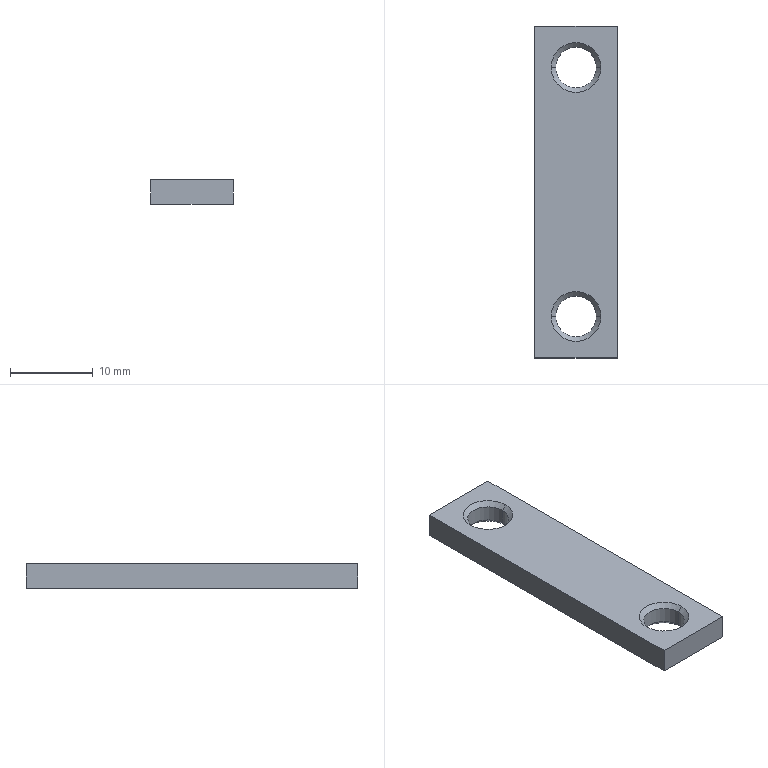Part | STEP file | hhpnt6_2_2_03 | 1 solid | 18 faces | box 10 x 40 x 3 mm | volume 1076 mm3 | cone 8 | plane 6 | cylinder 4 | commonest cylinder face diameters 4.917 x4
STEP:
#1=CARTESIAN_POINT('',(0.,0.,0.));
#2=DIRECTION('',(0.,0.,1.));
#3=DIRECTION('',(1.,0.,0.));
#4=AXIS2_PLACEMENT_3D('',#1,#2,#3);
#5=CARTESIAN_POINT('',(-2.459,-15.,0.5415));
#6=VERTEX_POINT('',#5);
#7=CARTESIAN_POINT('',(-3.,-15.,0.));
#8=VERTEX_POINT('',#7);
#9=CARTESIAN_POINT('',(-3.,-15.,0.));
#10=DIRECTION('',(-0.7071,0.,-0.7071));
#11=VECTOR('',#10,1.);
#12=LINE('',#9,#11);
#13=CARTESIAN_POINT('',(0.,-15.,0.));
#14=DIRECTION('',(0.,0.,-1.));
#15=DIRECTION('',(-1.,0.,0.));
#16=AXIS2_PLACEMENT_3D('',#13,#14,#15);
#17=CONICAL_SURFACE('',#16,3.,0.7854);
#18=CARTESIAN_POINT('',(6.283,0.));
#19=DIRECTION('',(0.,1.));
#20=VECTOR('',#19,1.);
#21=LINE('',#18,#20);
#22=(GEOMETRIC_REPRESENTATION_CONTEXT(2)PARAMETRIC_REPRESENTATION_CONTEXT()REPRESENTATION_CONTEXT('',''));
#23=DEFINITIONAL_REPRESENTATION('',(#21),#22);
#24=PCURVE('',#17,#23);
#25=CARTESIAN_POINT('',(0.,-15.,0.));
#26=DIRECTION('',(0.,0.,-1.));
#27=DIRECTION('',(-1.,0.,0.));
#28=AXIS2_PLACEMENT_3D('',#25,#26,#27);
#29=CONICAL_SURFACE('',#28,3.,0.7854);
#30=CARTESIAN_POINT('',(0.,0.));
#31=DIRECTION('',(0.,1.));
#32=VECTOR('',#31,1.);
#33=LINE('',#30,#32);
#34=(GEOMETRIC_REPRESENTATION_CONTEXT(2)PARAMETRIC_REPRESENTATION_CONTEXT()REPRESENTATION_CONTEXT('',''));
#35=DEFINITIONAL_REPRESENTATION('',(#33),#34);
#36=PCURVE('',#29,#35);
#37=SURFACE_CURVE('',#12,(#24,#36),.PCURVE_S1.);
#38=EDGE_CURVE('',#6,#8,#37,.T.);
#39=ORIENTED_EDGE('',*,*,#38,.T.);
#40=CARTESIAN_POINT('',(3.,-15.,0.));
#41=VERTEX_POINT('',#40);
#42=CARTESIAN_POINT('',(0.,-15.,0.));
#43=DIRECTION('',(0.,0.,-1.));
#44=DIRECTION('',(-1.,0.,0.));
#45=AXIS2_PLACEMENT_3D('',#42,#43,#44);
#46=CIRCLE('',#45,3.);
#47=CARTESIAN_POINT('',(0.,0.));
#48=DIRECTION('',(1.,0.));
#49=VECTOR('',#48,1.);
#50=LINE('',#47,#49);
#51=(GEOMETRIC_REPRESENTATION_CONTEXT(2)PARAMETRIC_REPRESENTATION_CONTEXT()REPRESENTATION_CONTEXT('',''));
#52=DEFINITIONAL_REPRESENTATION('',(#50),#51);
#53=PCURVE('',#17,#52);
#54=CARTESIAN_POINT('',(0.,0.,0.));
#55=DIRECTION('',(0.,0.,1.));
#56=DIRECTION('',(1.,0.,0.));
#57=AXIS2_PLACEMENT_3D('',#54,#55,#56);
#58=PLANE('',#57);
#59=CARTESIAN_POINT('',(-3.,-15.));
#60=CARTESIAN_POINT('',(-3.,-9.804));
#61=CARTESIAN_POINT('',(1.5,-12.402));
#62=CARTESIAN_POINT('',(6.,-15.));
#63=CARTESIAN_POINT('',(1.5,-17.598));
#64=CARTESIAN_POINT('',(-3.,-20.196));
#65=CARTESIAN_POINT('',(-3.,-15.));
#66=(BOUNDED_CURVE()B_SPLINE_CURVE(2,(#59,#60,#61,#62,#63,#64,#65),.UNSPECIFIED.,.T.,.F.)B_SPLINE_CURVE_WITH_KNOTS((1,2,2,2,2,1),(-2.094,0.,2.094,4.189,6.283,8.378),.UNSPECIFIED.)CURVE()GEOMETRIC_REPRESENTATION_ITEM()RATIONAL_B_SPLINE_CURVE((1.,0.5,1.,0.5,1.,0.5,1.))REPRESENTATION_ITEM(''));
#67=(GEOMETRIC_REPRESENTATION_CONTEXT(2)PARAMETRIC_REPRESENTATION_CONTEXT()REPRESENTATION_CONTEXT('',''));
#68=DEFINITIONAL_REPRESENTATION('',(#66),#67);
#69=PCURVE('',#58,#68);
#70=SURFACE_CURVE('',#46,(#53,#69),.PCURVE_S1.);
#71=EDGE_CURVE('',#41,#8,#70,.T.);
#72=ORIENTED_EDGE('',*,*,#71,.F.);
#73=CARTESIAN_POINT('',(2.459,-15.,0.5415));
#74=VERTEX_POINT('',#73);
#75=CARTESIAN_POINT('',(3.,-15.,0.));
#76=DIRECTION('',(0.7071,0.,-0.7071));
#77=VECTOR('',#76,1.);
#78=LINE('',#75,#77);
#79=CARTESIAN_POINT('',(3.142,0.));
#80=DIRECTION('',(0.,1.));
#81=VECTOR('',#80,1.);
#82=LINE('',#79,#81);
#83=(GEOMETRIC_REPRESENTATION_CONTEXT(2)PARAMETRIC_REPRESENTATION_CONTEXT()REPRESENTATION_CONTEXT('',''));
#84=DEFINITIONAL_REPRESENTATION('',(#82),#83);
#85=PCURVE('',#17,#84);
#86=CARTESIAN_POINT('',(3.142,0.));
#87=DIRECTION('',(0.,1.));
#88=VECTOR('',#87,1.);
#89=LINE('',#86,#88);
#90=(GEOMETRIC_REPRESENTATION_CONTEXT(2)PARAMETRIC_REPRESENTATION_CONTEXT()REPRESENTATION_CONTEXT('',''));
#91=DEFINITIONAL_REPRESENTATION('',(#89),#90);
#92=PCURVE('',#29,#91);
#93=SURFACE_CURVE('',#78,(#85,#92),.PCURVE_S1.);
#94=EDGE_CURVE('',#74,#41,#93,.T.);
#95=ORIENTED_EDGE('',*,*,#94,.F.);
#96=CARTESIAN_POINT('',(0.,-15.,0.5415));
#97=DIRECTION('',(0.,0.,-1.));
#98=DIRECTION('',(0.,-1.,0.));
#99=AXIS2_PLACEMENT_3D('',#96,#97,#98);
#100=CIRCLE('',#99,2.459);
#101=CARTESIAN_POINT('',(-1.571,-0.5415));
#102=DIRECTION('',(1.,0.));
#103=VECTOR('',#102,1.);
#104=LINE('',#101,#103);
#105=(GEOMETRIC_REPRESENTATION_CONTEXT(2)PARAMETRIC_REPRESENTATION_CONTEXT()REPRESENTATION_CONTEXT('',''));
#106=DEFINITIONAL_REPRESENTATION('',(#104),#105);
#107=PCURVE('',#17,#106);
#108=CARTESIAN_POINT('',(0.,-15.,1.5));
#109=DIRECTION('',(0.,0.,1.));
#110=DIRECTION('',(1.,0.,0.));
#111=AXIS2_PLACEMENT_3D('',#108,#109,#110);
#112=CYLINDRICAL_SURFACE('',#111,2.458);
#113=CARTESIAN_POINT('',(10.996,-0.9585));
#114=DIRECTION('',(-1.,0.));
#115=VECTOR('',#114,1.);
#116=LINE('',#113,#115);
#117=(GEOMETRIC_REPRESENTATION_CONTEXT(2)PARAMETRIC_REPRESENTATION_CONTEXT()REPRESENTATION_CONTEXT('',''));
#118=DEFINITIONAL_REPRESENTATION('',(#116),#117);
#119=PCURVE('',#112,#118);
#120=SURFACE_CURVE('',#100,(#107,#119),.PCURVE_S1.);
#121=EDGE_CURVE('',#74,#6,#120,.T.);
#122=ORIENTED_EDGE('',*,*,#121,.T.);
#123=EDGE_LOOP('',(#39,#72,#95,#122));
#124=FACE_BOUND('',#123,.F.);
#125=ADVANCED_FACE('',(#124),#17,.F.);
#126=CARTESIAN_POINT('',(-2.459,15.,0.5415));
#127=VERTEX_POINT('',#126);
#128=CARTESIAN_POINT('',(-3.,15.,0.));
#129=VERTEX_POINT('',#128);
#130=CARTESIAN_POINT('',(-3.,15.,0.));
#131=DIRECTION('',(-0.7071,0.,-0.7071));
#132=VECTOR('',#131,1.);
#133=LINE('',#130,#132);
#134=CARTESIAN_POINT('',(0.,15.,0.));
#135=DIRECTION('',(0.,0.,-1.));
#136=DIRECTION('',(-1.,0.,0.));
#137=AXIS2_PLACEMENT_3D('',#134,#135,#136);
#138=CONICAL_SURFACE('',#137,3.,0.7854);
#139=CARTESIAN_POINT('',(6.283,0.));
#140=DIRECTION('',(0.,1.));
#141=VECTOR('',#140,1.);
#142=LINE('',#139,#141);
#143=(GEOMETRIC_REPRESENTATION_CONTEXT(2)PARAMETRIC_REPRESENTATION_CONTEXT()REPRESENTATION_CONTEXT('',''));
#144=DEFINITIONAL_REPRESENTATION('',(#142),#143);
#145=PCURVE('',#138,#144);
#146=CARTESIAN_POINT('',(0.,15.,0.));
#147=DIRECTION('',(0.,0.,-1.));
#148=DIRECTION('',(-1.,0.,0.));
#149=AXIS2_PLACEMENT_3D('',#146,#147,#148);
#150=CONICAL_SURFACE('',#149,3.,0.7854);
#151=CARTESIAN_POINT('',(0.,0.));
#152=DIRECTION('',(0.,1.));
#153=VECTOR('',#152,1.);
#154=LINE('',#151,#153);
#155=(GEOMETRIC_REPRESENTATION_CONTEXT(2)PARAMETRIC_REPRESENTATION_CONTEXT()REPRESENTATION_CONTEXT('',''));
#156=DEFINITIONAL_REPRESENTATION('',(#154),#155);
#157=PCURVE('',#150,#156);
#158=SURFACE_CURVE('',#133,(#145,#157),.PCURVE_S1.);
#159=EDGE_CURVE('',#127,#129,#158,.T.);
#160=ORIENTED_EDGE('',*,*,#159,.T.);
#161=CARTESIAN_POINT('',(3.,15.,0.));
#162=VERTEX_POINT('',#161);
#163=CARTESIAN_POINT('',(0.,15.,0.));
#164=DIRECTION('',(0.,0.,-1.));
#165=DIRECTION('',(-1.,0.,0.));
#166=AXIS2_PLACEMENT_3D('',#163,#164,#165);
#167=CIRCLE('',#166,3.);
#168=CARTESIAN_POINT('',(0.,0.));
#169=DIRECTION('',(1.,0.));
#170=VECTOR('',#169,1.);
#171=LINE('',#168,#170);
#172=(GEOMETRIC_REPRESENTATION_CONTEXT(2)PARAMETRIC_REPRESENTATION_CONTEXT()REPRESENTATION_CONTEXT('',''));
#173=DEFINITIONAL_REPRESENTATION('',(#171),#172);
#174=PCURVE('',#138,#173);
#175=CARTESIAN_POINT('',(-3.,15.));
#176=CARTESIAN_POINT('',(-3.,20.196));
#177=CARTESIAN_POINT('',(1.5,17.598));
#178=CARTESIAN_POINT('',(6.,15.));
#179=CARTESIAN_POINT('',(1.5,12.402));
#180=CARTESIAN_POINT('',(-3.,9.804));
#181=CARTESIAN_POINT('',(-3.,15.));
#182=(BOUNDED_CURVE()B_SPLINE_CURVE(2,(#175,#176,#177,#178,#179,#180,#181),.UNSPECIFIED.,.T.,.F.)B_SPLINE_CURVE_WITH_KNOTS((1,2,2,2,2,1),(-2.094,0.,2.094,4.189,6.283,8.378),.UNSPECIFIED.)CURVE()GEOMETRIC_REPRESENTATION_ITEM()RATIONAL_B_SPLINE_CURVE((1.,0.5,1.,0.5,1.,0.5,1.))REPRESENTATION_ITEM(''));
#183=(GEOMETRIC_REPRESENTATION_CONTEXT(2)PARAMETRIC_REPRESENTATION_CONTEXT()REPRESENTATION_CONTEXT('',''));
#184=DEFINITIONAL_REPRESENTATION('',(#182),#183);
#185=PCURVE('',#58,#184);
#186=SURFACE_CURVE('',#167,(#174,#185),.PCURVE_S1.);
#187=EDGE_CURVE('',#162,#129,#186,.T.);
#188=ORIENTED_EDGE('',*,*,#187,.F.);
#189=CARTESIAN_POINT('',(2.459,15.,0.5415));
#190=VERTEX_POINT('',#189);
#191=CARTESIAN_POINT('',(3.,15.,0.));
#192=DIRECTION('',(0.7071,0.,-0.7071));
#193=VECTOR('',#192,1.);
#194=LINE('',#191,#193);
#195=CARTESIAN_POINT('',(3.142,0.));
#196=DIRECTION('',(0.,1.));
#197=VECTOR('',#196,1.);
#198=LINE('',#195,#197);
#199=(GEOMETRIC_REPRESENTATION_CONTEXT(2)PARAMETRIC_REPRESENTATION_CONTEXT()REPRESENTATION_CONTEXT('',''));
#200=DEFINITIONAL_REPRESENTATION('',(#198),#199);
#201=PCURVE('',#138,#200);
#202=CARTESIAN_POINT('',(3.142,0.));
#203=DIRECTION('',(0.,1.));
#204=VECTOR('',#203,1.);
#205=LINE('',#202,#204);
#206=(GEOMETRIC_REPRESENTATION_CONTEXT(2)PARAMETRIC_REPRESENTATION_CONTEXT()REPRESENTATION_CONTEXT('',''));
#207=DEFINITIONAL_REPRESENTATION('',(#205),#206);
#208=PCURVE('',#150,#207);
#209=SURFACE_CURVE('',#194,(#201,#208),.PCURVE_S1.);
#210=EDGE_CURVE('',#190,#162,#209,.T.);
#211=ORIENTED_EDGE('',*,*,#210,.F.);
#212=CARTESIAN_POINT('',(0.,15.,0.5415));
#213=DIRECTION('',(0.,0.,-1.));
#214=DIRECTION('',(0.,-1.,0.));
#215=AXIS2_PLACEMENT_3D('',#212,#213,#214);
#216=CIRCLE('',#215,2.459);
#217=CARTESIAN_POINT('',(-1.571,-0.5415));
#218=DIRECTION('',(1.,0.));
#219=VECTOR('',#218,1.);
#220=LINE('',#217,#219);
#221=(GEOMETRIC_REPRESENTATION_CONTEXT(2)PARAMETRIC_REPRESENTATION_CONTEXT()REPRESENTATION_CONTEXT('',''));
#222=DEFINITIONAL_REPRESENTATION('',(#220),#221);
#223=PCURVE('',#138,#222);
#224=CARTESIAN_POINT('',(0.,15.,1.5));
#225=DIRECTION('',(0.,0.,1.));
#226=DIRECTION('',(1.,0.,0.));
#227=AXIS2_PLACEMENT_3D('',#224,#225,#226);
#228=CYLINDRICAL_SURFACE('',#227,2.458);
#229=CARTESIAN_POINT('',(10.996,-0.9585));
#230=DIRECTION('',(-1.,0.));
#231=VECTOR('',#230,1.);
#232=LINE('',#229,#231);
#233=(GEOMETRIC_REPRESENTATION_CONTEXT(2)PARAMETRIC_REPRESENTATION_CONTEXT()REPRESENTATION_CONTEXT('',''));
#234=DEFINITIONAL_REPRESENTATION('',(#232),#233);
#235=PCURVE('',#228,#234);
#236=SURFACE_CURVE('',#216,(#223,#235),.PCURVE_S1.);
#237=EDGE_CURVE('',#190,#127,#236,.T.);
#238=ORIENTED_EDGE('',*,*,#237,.T.);
#239=EDGE_LOOP('',(#160,#188,#211,#238));
#240=FACE_BOUND('',#239,.F.);
#241=ADVANCED_FACE('',(#240),#138,.F.);
#242=CARTESIAN_POINT('',(2.458,-15.,2.458));
#243=VERTEX_POINT('',#242);
#244=CARTESIAN_POINT('',(2.458,-15.,1.5));
#245=DIRECTION('',(0.,0.,1.));
#246=VECTOR('',#245,1.);
#247=LINE('',#244,#246);
#248=CARTESIAN_POINT('',(6.283,0.));
#249=DIRECTION('',(0.,1.));
#250=VECTOR('',#249,1.);
#251=LINE('',#248,#250);
#252=(GEOMETRIC_REPRESENTATION_CONTEXT(2)PARAMETRIC_REPRESENTATION_CONTEXT()REPRESENTATION_CONTEXT('',''));
#253=DEFINITIONAL_REPRESENTATION('',(#251),#252);
#254=PCURVE('',#112,#253);
#255=CARTESIAN_POINT('',(0.,-15.,1.5));
#256=DIRECTION('',(0.,0.,1.));
#257=DIRECTION('',(1.,0.,0.));
#258=AXIS2_PLACEMENT_3D('',#255,#256,#257);
#259=CYLINDRICAL_SURFACE('',#258,2.458);
#260=CARTESIAN_POINT('',(0.,0.));
#261=DIRECTION('',(0.,1.));
#262=VECTOR('',#261,1.);
#263=LINE('',#260,#262);
#264=(GEOMETRIC_REPRESENTATION_CONTEXT(2)PARAMETRIC_REPRESENTATION_CONTEXT()REPRESENTATION_CONTEXT('',''));
#265=DEFINITIONAL_REPRESENTATION('',(#263),#264);
#266=PCURVE('',#259,#265);
#267=SURFACE_CURVE('',#247,(#254,#266),.PCURVE_S1.);
#268=EDGE_CURVE('',#74,#243,#267,.T.);
#269=ORIENTED_EDGE('',*,*,#268,.T.);
#270=CARTESIAN_POINT('',(-2.458,-15.,2.458));
#271=VERTEX_POINT('',#270);
#272=CARTESIAN_POINT('',(0.,-15.,2.458));
#273=DIRECTION('',(0.,0.,-1.));
#274=DIRECTION('',(1.,0.,0.));
#275=AXIS2_PLACEMENT_3D('',#272,#273,#274);
#276=CIRCLE('',#275,2.458);
#277=CARTESIAN_POINT('',(6.283,0.9585));
#278=DIRECTION('',(-1.,0.));
#279=VECTOR('',#278,1.);
#280=LINE('',#277,#279);
#281=(GEOMETRIC_REPRESENTATION_CONTEXT(2)PARAMETRIC_REPRESENTATION_CONTEXT()REPRESENTATION_CONTEXT('',''));
#282=DEFINITIONAL_REPRESENTATION('',(#280),#281);
#283=PCURVE('',#112,#282);
#284=CARTESIAN_POINT('',(0.,-15.,3.));
#285=DIRECTION('',(0.,0.,1.));
#286=DIRECTION('',(1.,0.,0.));
#287=AXIS2_PLACEMENT_3D('',#284,#285,#286);
#288=CONICAL_SURFACE('',#287,3.,0.7854);
#289=CARTESIAN_POINT('',(6.283,-0.5415));
#290=DIRECTION('',(-1.,0.));
#291=VECTOR('',#290,1.);
#292=LINE('',#289,#291);
#293=(GEOMETRIC_REPRESENTATION_CONTEXT(2)PARAMETRIC_REPRESENTATION_CONTEXT()REPRESENTATION_CONTEXT('',''));
#294=DEFINITIONAL_REPRESENTATION('',(#292),#293);
#295=PCURVE('',#288,#294);
#296=SURFACE_CURVE('',#276,(#283,#295),.PCURVE_S1.);
#297=EDGE_CURVE('',#243,#271,#296,.T.);
#298=ORIENTED_EDGE('',*,*,#297,.T.);
#299=CARTESIAN_POINT('',(-2.458,-15.,1.5));
#300=DIRECTION('',(0.,0.,1.));
#301=VECTOR('',#300,1.);
#302=LINE('',#299,#301);
#303=CARTESIAN_POINT('',(3.142,0.));
#304=DIRECTION('',(0.,1.));
#305=VECTOR('',#304,1.);
#306=LINE('',#303,#305);
#307=(GEOMETRIC_REPRESENTATION_CONTEXT(2)PARAMETRIC_REPRESENTATION_CONTEXT()REPRESENTATION_CONTEXT('',''));
#308=DEFINITIONAL_REPRESENTATION('',(#306),#307);
#309=PCURVE('',#112,#308);
#310=CARTESIAN_POINT('',(3.142,0.));
#311=DIRECTION('',(0.,1.));
#312=VECTOR('',#311,1.);
#313=LINE('',#310,#312);
#314=(GEOMETRIC_REPRESENTATION_CONTEXT(2)PARAMETRIC_REPRESENTATION_CONTEXT()REPRESENTATION_CONTEXT('',''));
#315=DEFINITIONAL_REPRESENTATION('',(#313),#314);
#316=PCURVE('',#259,#315);
#317=SURFACE_CURVE('',#302,(#309,#316),.PCURVE_S1.);
#318=EDGE_CURVE('',#6,#271,#317,.T.);
#319=ORIENTED_EDGE('',*,*,#318,.F.);
#320=ORIENTED_EDGE('',*,*,#121,.F.);
#321=EDGE_LOOP('',(#269,#298,#319,#320));
#322=FACE_BOUND('',#321,.F.);
#323=ADVANCED_FACE('',(#322),#112,.F.);
#324=CARTESIAN_POINT('',(2.458,15.,2.458));
#325=VERTEX_POINT('',#324);
#326=CARTESIAN_POINT('',(2.458,15.,1.5));
#327=DIRECTION('',(0.,0.,1.));
#328=VECTOR('',#327,1.);
#329=LINE('',#326,#328);
#330=CARTESIAN_POINT('',(6.283,0.));
#331=DIRECTION('',(0.,1.));
#332=VECTOR('',#331,1.);
#333=LINE('',#330,#332);
#334=(GEOMETRIC_REPRESENTATION_CONTEXT(2)PARAMETRIC_REPRESENTATION_CONTEXT()REPRESENTATION_CONTEXT('',''));
#335=DEFINITIONAL_REPRESENTATION('',(#333),#334);
#336=PCURVE('',#228,#335);
#337=CARTESIAN_POINT('',(0.,15.,1.5));
#338=DIRECTION('',(0.,0.,1.));
#339=DIRECTION('',(1.,0.,0.));
#340=AXIS2_PLACEMENT_3D('',#337,#338,#339);
#341=CYLINDRICAL_SURFACE('',#340,2.458);
#342=CARTESIAN_POINT('',(0.,0.));
#343=DIRECTION('',(0.,1.));
#344=VECTOR('',#343,1.);
#345=LINE('',#342,#344);
#346=(GEOMETRIC_REPRESENTATION_CONTEXT(2)PARAMETRIC_REPRESENTATION_CONTEXT()REPRESENTATION_CONTEXT('',''));
#347=DEFINITIONAL_REPRESENTATION('',(#345),#346);
#348=PCURVE('',#341,#347);
#349=SURFACE_CURVE('',#329,(#336,#348),.PCURVE_S1.);
#350=EDGE_CURVE('',#190,#325,#349,.T.);
#351=ORIENTED_EDGE('',*,*,#350,.T.);
#352=CARTESIAN_POINT('',(-2.458,15.,2.458));
#353=VERTEX_POINT('',#352);
#354=CARTESIAN_POINT('',(0.,15.,2.458));
#355=DIRECTION('',(0.,0.,-1.));
#356=DIRECTION('',(1.,0.,0.));
#357=AXIS2_PLACEMENT_3D('',#354,#355,#356);
#358=CIRCLE('',#357,2.458);
#359=CARTESIAN_POINT('',(6.283,0.9585));
#360=DIRECTION('',(-1.,0.));
#361=VECTOR('',#360,1.);
#362=LINE('',#359,#361);
#363=(GEOMETRIC_REPRESENTATION_CONTEXT(2)PARAMETRIC_REPRESENTATION_CONTEXT()REPRESENTATION_CONTEXT('',''));
#364=DEFINITIONAL_REPRESENTATION('',(#362),#363);
#365=PCURVE('',#228,#364);
#366=CARTESIAN_POINT('',(0.,15.,3.));
#367=DIRECTION('',(0.,0.,1.));
#368=DIRECTION('',(1.,0.,0.));
#369=AXIS2_PLACEMENT_3D('',#366,#367,#368);
#370=CONICAL_SURFACE('',#369,3.,0.7854);
#371=CARTESIAN_POINT('',(6.283,-0.5415));
#372=DIRECTION('',(-1.,0.));
#373=VECTOR('',#372,1.);
#374=LINE('',#371,#373);
#375=(GEOMETRIC_REPRESENTATION_CONTEXT(2)PARAMETRIC_REPRESENTATION_CONTEXT()REPRESENTATION_CONTEXT('',''));
#376=DEFINITIONAL_REPRESENTATION('',(#374),#375);
#377=PCURVE('',#370,#376);
#378=SURFACE_CURVE('',#358,(#365,#377),.PCURVE_S1.);
#379=EDGE_CURVE('',#325,#353,#378,.T.);
#380=ORIENTED_EDGE('',*,*,#379,.T.);
#381=CARTESIAN_POINT('',(-2.458,15.,1.5));
#382=DIRECTION('',(0.,0.,1.));
#383=VECTOR('',#382,1.);
#384=LINE('',#381,#383);
#385=CARTESIAN_POINT('',(3.142,0.));
#386=DIRECTION('',(0.,1.));
#387=VECTOR('',#386,1.);
#388=LINE('',#385,#387);
#389=(GEOMETRIC_REPRESENTATION_CONTEXT(2)PARAMETRIC_REPRESENTATION_CONTEXT()REPRESENTATION_CONTEXT('',''));
#390=DEFINITIONAL_REPRESENTATION('',(#388),#389);
#391=PCURVE('',#228,#390);
#392=CARTESIAN_POINT('',(3.142,0.));
#393=DIRECTION('',(0.,1.));
#394=VECTOR('',#393,1.);
#395=LINE('',#392,#394);
#396=(GEOMETRIC_REPRESENTATION_CONTEXT(2)PARAMETRIC_REPRESENTATION_CONTEXT()REPRESENTATION_CONTEXT('',''));
#397=DEFINITIONAL_REPRESENTATION('',(#395),#396);
#398=PCURVE('',#341,#397);
#399=SURFACE_CURVE('',#384,(#391,#398),.PCURVE_S1.);
#400=EDGE_CURVE('',#127,#353,#399,.T.);
#401=ORIENTED_EDGE('',*,*,#400,.F.);
#402=ORIENTED_EDGE('',*,*,#237,.F.);
#403=EDGE_LOOP('',(#351,#380,#401,#402));
#404=FACE_BOUND('',#403,.F.);
#405=ADVANCED_FACE('',(#404),#228,.F.);
#406=CARTESIAN_POINT('',(3.,-15.,3.));
#407=VERTEX_POINT('',#406);
#408=CARTESIAN_POINT('',(3.,-15.,3.));
#409=DIRECTION('',(0.7071,0.,0.7071));
#410=VECTOR('',#409,1.);
#411=LINE('',#408,#410);
#412=CARTESIAN_POINT('',(6.283,0.));
#413=DIRECTION('',(0.,1.));
#414=VECTOR('',#413,1.);
#415=LINE('',#412,#414);
#416=(GEOMETRIC_REPRESENTATION_CONTEXT(2)PARAMETRIC_REPRESENTATION_CONTEXT()REPRESENTATION_CONTEXT('',''));
#417=DEFINITIONAL_REPRESENTATION('',(#415),#416);
#418=PCURVE('',#288,#417);
#419=CARTESIAN_POINT('',(0.,-15.,3.));
#420=DIRECTION('',(0.,0.,1.));
#421=DIRECTION('',(1.,0.,0.));
#422=AXIS2_PLACEMENT_3D('',#419,#420,#421);
#423=CONICAL_SURFACE('',#422,3.,0.7854);
#424=CARTESIAN_POINT('',(0.,0.));
#425=DIRECTION('',(0.,1.));
#426=VECTOR('',#425,1.);
#427=LINE('',#424,#426);
#428=(GEOMETRIC_REPRESENTATION_CONTEXT(2)PARAMETRIC_REPRESENTATION_CONTEXT()REPRESENTATION_CONTEXT('',''));
#429=DEFINITIONAL_REPRESENTATION('',(#427),#428);
#430=PCURVE('',#423,#429);
#431=SURFACE_CURVE('',#411,(#418,#430),.PCURVE_S1.);
#432=EDGE_CURVE('',#243,#407,#431,.T.);
#433=ORIENTED_EDGE('',*,*,#432,.T.);
#434=CARTESIAN_POINT('',(-3.,-15.,3.));
#435=VERTEX_POINT('',#434);
#436=CARTESIAN_POINT('',(0.,-15.,3.));
#437=DIRECTION('',(0.,0.,-1.));
#438=DIRECTION('',(1.,0.,0.));
#439=AXIS2_PLACEMENT_3D('',#436,#437,#438);
#440=CIRCLE('',#439,3.);
#441=CARTESIAN_POINT('',(6.283,0.));
#442=DIRECTION('',(-1.,0.));
#443=VECTOR('',#442,1.);
#444=LINE('',#441,#443);
#445=(GEOMETRIC_REPRESENTATION_CONTEXT(2)PARAMETRIC_REPRESENTATION_CONTEXT()REPRESENTATION_CONTEXT('',''));
#446=DEFINITIONAL_REPRESENTATION('',(#444),#445);
#447=PCURVE('',#288,#446);
#448=CARTESIAN_POINT('',(0.,0.,3.));
#449=DIRECTION('',(0.,0.,1.));
#450=DIRECTION('',(1.,0.,0.));
#451=AXIS2_PLACEMENT_3D('',#448,#449,#450);
#452=PLANE('',#451);
#453=CARTESIAN_POINT('',(3.,-15.));
#454=CARTESIAN_POINT('',(3.,-20.196));
#455=CARTESIAN_POINT('',(-1.5,-17.598));
#456=CARTESIAN_POINT('',(-6.,-15.));
#457=CARTESIAN_POINT('',(-1.5,-12.402));
#458=CARTESIAN_POINT('',(3.,-9.804));
#459=CARTESIAN_POINT('',(3.,-15.));
#460=(BOUNDED_CURVE()B_SPLINE_CURVE(2,(#453,#454,#455,#456,#457,#458,#459),.UNSPECIFIED.,.T.,.F.)B_SPLINE_CURVE_WITH_KNOTS((1,2,2,2,2,1),(-2.094,0.,2.094,4.189,6.283,8.378),.UNSPECIFIED.)CURVE()GEOMETRIC_REPRESENTATION_ITEM()RATIONAL_B_SPLINE_CURVE((1.,0.5,1.,0.5,1.,0.5,1.))REPRESENTATION_ITEM(''));
#461=(GEOMETRIC_REPRESENTATION_CONTEXT(2)PARAMETRIC_REPRESENTATION_CONTEXT()REPRESENTATION_CONTEXT('',''));
#462=DEFINITIONAL_REPRESENTATION('',(#460),#461);
#463=PCURVE('',#452,#462);
#464=SURFACE_CURVE('',#440,(#447,#463),.PCURVE_S1.);
#465=EDGE_CURVE('',#407,#435,#464,.T.);
#466=ORIENTED_EDGE('',*,*,#465,.T.);
#467=CARTESIAN_POINT('',(-3.,-15.,3.));
#468=DIRECTION('',(-0.7071,0.,0.7071));
#469=VECTOR('',#468,1.);
#470=LINE('',#467,#469);
#471=CARTESIAN_POINT('',(3.142,0.));
#472=DIRECTION('',(0.,1.));
#473=VECTOR('',#472,1.);
#474=LINE('',#471,#473);
#475=(GEOMETRIC_REPRESENTATION_CONTEXT(2)PARAMETRIC_REPRESENTATION_CONTEXT()REPRESENTATION_CONTEXT('',''));
#476=DEFINITIONAL_REPRESENTATION('',(#474),#475);
#477=PCURVE('',#288,#476);
#478=CARTESIAN_POINT('',(3.142,0.));
#479=DIRECTION('',(0.,1.));
#480=VECTOR('',#479,1.);
#481=LINE('',#478,#480);
#482=(GEOMETRIC_REPRESENTATION_CONTEXT(2)PARAMETRIC_REPRESENTATION_CONTEXT()REPRESENTATION_CONTEXT('',''));
#483=DEFINITIONAL_REPRESENTATION('',(#481),#482);
#484=PCURVE('',#423,#483);
#485=SURFACE_CURVE('',#470,(#477,#484),.PCURVE_S1.);
#486=EDGE_CURVE('',#271,#435,#485,.T.);
#487=ORIENTED_EDGE('',*,*,#486,.F.);
#488=ORIENTED_EDGE('',*,*,#297,.F.);
#489=EDGE_LOOP('',(#433,#466,#487,#488));
#490=FACE_BOUND('',#489,.F.);
#491=ADVANCED_FACE('',(#490),#288,.F.);
#492=CARTESIAN_POINT('',(3.,15.,3.));
#493=VERTEX_POINT('',#492);
#494=CARTESIAN_POINT('',(3.,15.,3.));
#495=DIRECTION('',(0.7071,0.,0.7071));
#496=VECTOR('',#495,1.);
#497=LINE('',#494,#496);
#498=CARTESIAN_POINT('',(6.283,0.));
#499=DIRECTION('',(0.,1.));
#500=VECTOR('',#499,1.);
#501=LINE('',#498,#500);
#502=(GEOMETRIC_REPRESENTATION_CONTEXT(2)PARAMETRIC_REPRESENTATION_CONTEXT()REPRESENTATION_CONTEXT('',''));
#503=DEFINITIONAL_REPRESENTATION('',(#501),#502);
#504=PCURVE('',#370,#503);
#505=CARTESIAN_POINT('',(0.,15.,3.));
#506=DIRECTION('',(0.,0.,1.));
#507=DIRECTION('',(1.,0.,0.));
#508=AXIS2_PLACEMENT_3D('',#505,#506,#507);
#509=CONICAL_SURFACE('',#508,3.,0.7854);
#510=CARTESIAN_POINT('',(0.,0.));
#511=DIRECTION('',(0.,1.));
#512=VECTOR('',#511,1.);
#513=LINE('',#510,#512);
#514=(GEOMETRIC_REPRESENTATION_CONTEXT(2)PARAMETRIC_REPRESENTATION_CONTEXT()REPRESENTATION_CONTEXT('',''));
#515=DEFINITIONAL_REPRESENTATION('',(#513),#514);
#516=PCURVE('',#509,#515);
#517=SURFACE_CURVE('',#497,(#504,#516),.PCURVE_S1.);
#518=EDGE_CURVE('',#325,#493,#517,.T.);
#519=ORIENTED_EDGE('',*,*,#518,.T.);
#520=CARTESIAN_POINT('',(-3.,15.,3.));
#521=VERTEX_POINT('',#520);
#522=CARTESIAN_POINT('',(0.,15.,3.));
#523=DIRECTION('',(0.,0.,-1.));
#524=DIRECTION('',(1.,0.,0.));
#525=AXIS2_PLACEMENT_3D('',#522,#523,#524);
#526=CIRCLE('',#525,3.);
#527=CARTESIAN_POINT('',(6.283,0.));
#528=DIRECTION('',(-1.,0.));
#529=VECTOR('',#528,1.);
#530=LINE('',#527,#529);
#531=(GEOMETRIC_REPRESENTATION_CONTEXT(2)PARAMETRIC_REPRESENTATION_CONTEXT()REPRESENTATION_CONTEXT('',''));
#532=DEFINITIONAL_REPRESENTATION('',(#530),#531);
#533=PCURVE('',#370,#532);
#534=CARTESIAN_POINT('',(3.,15.));
#535=CARTESIAN_POINT('',(3.,9.804));
#536=CARTESIAN_POINT('',(-1.5,12.402));
#537=CARTESIAN_POINT('',(-6.,15.));
#538=CARTESIAN_POINT('',(-1.5,17.598));
#539=CARTESIAN_POINT('',(3.,20.196));
#540=CARTESIAN_POINT('',(3.,15.));
#541=(BOUNDED_CURVE()B_SPLINE_CURVE(2,(#534,#535,#536,#537,#538,#539,#540),.UNSPECIFIED.,.T.,.F.)B_SPLINE_CURVE_WITH_KNOTS((1,2,2,2,2,1),(-2.094,0.,2.094,4.189,6.283,8.378),.UNSPECIFIED.)CURVE()GEOMETRIC_REPRESENTATION_ITEM()RATIONAL_B_SPLINE_CURVE((1.,0.5,1.,0.5,1.,0.5,1.))REPRESENTATION_ITEM(''));
#542=(GEOMETRIC_REPRESENTATION_CONTEXT(2)PARAMETRIC_REPRESENTATION_CONTEXT()REPRESENTATION_CONTEXT('',''));
#543=DEFINITIONAL_REPRESENTATION('',(#541),#542);
#544=PCURVE('',#452,#543);
#545=SURFACE_CURVE('',#526,(#533,#544),.PCURVE_S1.);
#546=EDGE_CURVE('',#493,#521,#545,.T.);
#547=ORIENTED_EDGE('',*,*,#546,.T.);
#548=CARTESIAN_POINT('',(-3.,15.,3.));
#549=DIRECTION('',(-0.7071,0.,0.7071));
#550=VECTOR('',#549,1.);
#551=LINE('',#548,#550);
#552=CARTESIAN_POINT('',(3.142,0.));
#553=DIRECTION('',(0.,1.));
#554=VECTOR('',#553,1.);
#555=LINE('',#552,#554);
#556=(GEOMETRIC_REPRESENTATION_CONTEXT(2)PARAMETRIC_REPRESENTATION_CONTEXT()REPRESENTATION_CONTEXT('',''));
#557=DEFINITIONAL_REPRESENTATION('',(#555),#556);
#558=PCURVE('',#370,#557);
#559=CARTESIAN_POINT('',(3.142,0.));
#560=DIRECTION('',(0.,1.));
#561=VECTOR('',#560,1.);
#562=LINE('',#559,#561);
#563=(GEOMETRIC_REPRESENTATION_CONTEXT(2)PARAMETRIC_REPRESENTATION_CONTEXT()REPRESENTATION_CONTEXT('',''));
#564=DEFINITIONAL_REPRESENTATION('',(#562),#563);
#565=PCURVE('',#509,#564);
#566=SURFACE_CURVE('',#551,(#558,#565),.PCURVE_S1.);
#567=EDGE_CURVE('',#353,#521,#566,.T.);
#568=ORIENTED_EDGE('',*,*,#567,.F.);
#569=ORIENTED_EDGE('',*,*,#379,.F.);
#570=EDGE_LOOP('',(#519,#547,#568,#569));
#571=FACE_BOUND('',#570,.F.);
#572=ADVANCED_FACE('',(#571),#370,.F.);
#573=CARTESIAN_POINT('',(5.,20.,0.));
#574=VERTEX_POINT('',#573);
#575=CARTESIAN_POINT('',(-5.,20.,0.));
#576=VERTEX_POINT('',#575);
#577=CARTESIAN_POINT('',(0.,20.,0.));
#578=DIRECTION('',(-1.,0.,0.));
#579=VECTOR('',#578,1.);
#580=LINE('',#577,#579);
#581=CARTESIAN_POINT('',(0.,20.));
#582=DIRECTION('',(-1.,0.));
#583=VECTOR('',#582,1.);
#584=LINE('',#581,#583);
#585=(GEOMETRIC_REPRESENTATION_CONTEXT(2)PARAMETRIC_REPRESENTATION_CONTEXT()REPRESENTATION_CONTEXT('',''));
#586=DEFINITIONAL_REPRESENTATION('',(#584),#585);
#587=PCURVE('',#58,#586);
#588=CARTESIAN_POINT('',(-5.,20.,0.));
#589=DIRECTION('',(0.,1.,0.));
#590=DIRECTION('',(0.,0.,1.));
#591=AXIS2_PLACEMENT_3D('',#588,#589,#590);
#592=PLANE('',#591);
#593=CARTESIAN_POINT('',(0.,5.));
#594=DIRECTION('',(0.,-1.));
#595=VECTOR('',#594,1.);
#596=LINE('',#593,#595);
#597=(GEOMETRIC_REPRESENTATION_CONTEXT(2)PARAMETRIC_REPRESENTATION_CONTEXT()REPRESENTATION_CONTEXT('',''));
#598=DEFINITIONAL_REPRESENTATION('',(#596),#597);
#599=PCURVE('',#592,#598);
#600=SURFACE_CURVE('',#580,(#587,#599),.PCURVE_S1.);
#601=EDGE_CURVE('',#574,#576,#600,.T.);
#602=ORIENTED_EDGE('',*,*,#601,.F.);
#603=CARTESIAN_POINT('',(5.,-20.,0.));
#604=VERTEX_POINT('',#603);
#605=CARTESIAN_POINT('',(5.,0.,0.));
#606=DIRECTION('',(0.,1.,0.));
#607=VECTOR('',#606,1.);
#608=LINE('',#605,#607);
#609=CARTESIAN_POINT('',(5.,0.));
#610=DIRECTION('',(0.,1.));
#611=VECTOR('',#610,1.);
#612=LINE('',#609,#611);
#613=(GEOMETRIC_REPRESENTATION_CONTEXT(2)PARAMETRIC_REPRESENTATION_CONTEXT()REPRESENTATION_CONTEXT('',''));
#614=DEFINITIONAL_REPRESENTATION('',(#612),#613);
#615=PCURVE('',#58,#614);
#616=CARTESIAN_POINT('',(5.,20.,0.));
#617=DIRECTION('',(1.,0.,0.));
#618=DIRECTION('',(0.,0.,-1.));
#619=AXIS2_PLACEMENT_3D('',#616,#617,#618);
#620=PLANE('',#619);
#621=CARTESIAN_POINT('',(0.,-20.));
#622=DIRECTION('',(0.,1.));
#623=VECTOR('',#622,1.);
#624=LINE('',#621,#623);
#625=(GEOMETRIC_REPRESENTATION_CONTEXT(2)PARAMETRIC_REPRESENTATION_CONTEXT()REPRESENTATION_CONTEXT('',''));
#626=DEFINITIONAL_REPRESENTATION('',(#624),#625);
#627=PCURVE('',#620,#626);
#628=SURFACE_CURVE('',#608,(#615,#627),.PCURVE_S1.);
#629=EDGE_CURVE('',#604,#574,#628,.T.);
#630=ORIENTED_EDGE('',*,*,#629,.F.);
#631=CARTESIAN_POINT('',(-5.,-20.,0.));
#632=VERTEX_POINT('',#631);
#633=CARTESIAN_POINT('',(0.,-20.,0.));
#634=DIRECTION('',(1.,0.,0.));
#635=VECTOR('',#634,1.);
#636=LINE('',#633,#635);
#637=CARTESIAN_POINT('',(0.,-20.));
#638=DIRECTION('',(1.,0.));
#639=VECTOR('',#638,1.);
#640=LINE('',#637,#639);
#641=(GEOMETRIC_REPRESENTATION_CONTEXT(2)PARAMETRIC_REPRESENTATION_CONTEXT()REPRESENTATION_CONTEXT('',''));
#642=DEFINITIONAL_REPRESENTATION('',(#640),#641);
#643=PCURVE('',#58,#642);
#644=CARTESIAN_POINT('',(5.,-20.,0.));
#645=DIRECTION('',(0.,-1.,0.));
#646=DIRECTION('',(0.,0.,-1.));
#647=AXIS2_PLACEMENT_3D('',#644,#645,#646);
#648=PLANE('',#647);
#649=CARTESIAN_POINT('',(0.,-5.));
#650=DIRECTION('',(0.,1.));
#651=VECTOR('',#650,1.);
#652=LINE('',#649,#651);
#653=(GEOMETRIC_REPRESENTATION_CONTEXT(2)PARAMETRIC_REPRESENTATION_CONTEXT()REPRESENTATION_CONTEXT('',''));
#654=DEFINITIONAL_REPRESENTATION('',(#652),#653);
#655=PCURVE('',#648,#654);
#656=SURFACE_CURVE('',#636,(#643,#655),.PCURVE_S1.);
#657=EDGE_CURVE('',#632,#604,#656,.T.);
#658=ORIENTED_EDGE('',*,*,#657,.F.);
#659=CARTESIAN_POINT('',(-5.,0.,0.));
#660=DIRECTION('',(0.,-1.,0.));
#661=VECTOR('',#660,1.);
#662=LINE('',#659,#661);
#663=CARTESIAN_POINT('',(-5.,0.));
#664=DIRECTION('',(0.,-1.));
#665=VECTOR('',#664,1.);
#666=LINE('',#663,#665);
#667=(GEOMETRIC_REPRESENTATION_CONTEXT(2)PARAMETRIC_REPRESENTATION_CONTEXT()REPRESENTATION_CONTEXT('',''));
#668=DEFINITIONAL_REPRESENTATION('',(#666),#667);
#669=PCURVE('',#58,#668);
#670=CARTESIAN_POINT('',(-5.,-20.,0.));
#671=DIRECTION('',(-1.,0.,0.));
#672=DIRECTION('',(0.,0.,1.));
#673=AXIS2_PLACEMENT_3D('',#670,#671,#672);
#674=PLANE('',#673);
#675=CARTESIAN_POINT('',(0.,20.));
#676=DIRECTION('',(0.,-1.));
#677=VECTOR('',#676,1.);
#678=LINE('',#675,#677);
#679=(GEOMETRIC_REPRESENTATION_CONTEXT(2)PARAMETRIC_REPRESENTATION_CONTEXT()REPRESENTATION_CONTEXT('',''));
#680=DEFINITIONAL_REPRESENTATION('',(#678),#679);
#681=PCURVE('',#674,#680);
#682=SURFACE_CURVE('',#662,(#669,#681),.PCURVE_S1.);
#683=EDGE_CURVE('',#576,#632,#682,.T.);
#684=ORIENTED_EDGE('',*,*,#683,.F.);
#685=EDGE_LOOP('',(#602,#630,#658,#684));
#686=FACE_BOUND('',#685,.T.);
#687=CARTESIAN_POINT('',(0.,-15.,0.));
#688=DIRECTION('',(0.,0.,-1.));
#689=DIRECTION('',(-1.,0.,0.));
#690=AXIS2_PLACEMENT_3D('',#687,#688,#689);
#691=CIRCLE('',#690,3.);
#692=CARTESIAN_POINT('',(-3.,-15.));
#693=CARTESIAN_POINT('',(-3.,-9.804));
#694=CARTESIAN_POINT('',(1.5,-12.402));
#695=CARTESIAN_POINT('',(6.,-15.));
#696=CARTESIAN_POINT('',(1.5,-17.598));
#697=CARTESIAN_POINT('',(-3.,-20.196));
#698=CARTESIAN_POINT('',(-3.,-15.));
#699=(BOUNDED_CURVE()B_SPLINE_CURVE(2,(#692,#693,#694,#695,#696,#697,#698),.UNSPECIFIED.,.T.,.F.)B_SPLINE_CURVE_WITH_KNOTS((1,2,2,2,2,1),(-2.094,0.,2.094,4.189,6.283,8.378),.UNSPECIFIED.)CURVE()GEOMETRIC_REPRESENTATION_ITEM()RATIONAL_B_SPLINE_CURVE((1.,0.5,1.,0.5,1.,0.5,1.))REPRESENTATION_ITEM(''));
#700=(GEOMETRIC_REPRESENTATION_CONTEXT(2)PARAMETRIC_REPRESENTATION_CONTEXT()REPRESENTATION_CONTEXT('',''));
#701=DEFINITIONAL_REPRESENTATION('',(#699),#700);
#702=PCURVE('',#58,#701);
#703=CARTESIAN_POINT('',(0.,0.));
#704=DIRECTION('',(1.,0.));
#705=VECTOR('',#704,1.);
#706=LINE('',#703,#705);
#707=(GEOMETRIC_REPRESENTATION_CONTEXT(2)PARAMETRIC_REPRESENTATION_CONTEXT()REPRESENTATION_CONTEXT('',''));
#708=DEFINITIONAL_REPRESENTATION('',(#706),#707);
#709=PCURVE('',#29,#708);
#710=SURFACE_CURVE('',#691,(#702,#709),.PCURVE_S1.);
#711=EDGE_CURVE('',#8,#41,#710,.T.);
#712=ORIENTED_EDGE('',*,*,#711,.F.);
#713=ORIENTED_EDGE('',*,*,#71,.F.);
#714=EDGE_LOOP('',(#712,#713));
#715=FACE_BOUND('',#714,.T.);
#716=CARTESIAN_POINT('',(0.,15.,0.));
#717=DIRECTION('',(0.,0.,-1.));
#718=DIRECTION('',(-1.,0.,0.));
#719=AXIS2_PLACEMENT_3D('',#716,#717,#718);
#720=CIRCLE('',#719,3.);
#721=CARTESIAN_POINT('',(-3.,15.));
#722=CARTESIAN_POINT('',(-3.,20.196));
#723=CARTESIAN_POINT('',(1.5,17.598));
#724=CARTESIAN_POINT('',(6.,15.));
#725=CARTESIAN_POINT('',(1.5,12.402));
#726=CARTESIAN_POINT('',(-3.,9.804));
#727=CARTESIAN_POINT('',(-3.,15.));
#728=(BOUNDED_CURVE()B_SPLINE_CURVE(2,(#721,#722,#723,#724,#725,#726,#727),.UNSPECIFIED.,.T.,.F.)B_SPLINE_CURVE_WITH_KNOTS((1,2,2,2,2,1),(-2.094,0.,2.094,4.189,6.283,8.378),.UNSPECIFIED.)CURVE()GEOMETRIC_REPRESENTATION_ITEM()RATIONAL_B_SPLINE_CURVE((1.,0.5,1.,0.5,1.,0.5,1.))REPRESENTATION_ITEM(''));
#729=(GEOMETRIC_REPRESENTATION_CONTEXT(2)PARAMETRIC_REPRESENTATION_CONTEXT()REPRESENTATION_CONTEXT('',''));
#730=DEFINITIONAL_REPRESENTATION('',(#728),#729);
#731=PCURVE('',#58,#730);
#732=CARTESIAN_POINT('',(0.,0.));
#733=DIRECTION('',(1.,0.));
#734=VECTOR('',#733,1.);
#735=LINE('',#732,#734);
#736=(GEOMETRIC_REPRESENTATION_CONTEXT(2)PARAMETRIC_REPRESENTATION_CONTEXT()REPRESENTATION_CONTEXT('',''));
#737=DEFINITIONAL_REPRESENTATION('',(#735),#736);
#738=PCURVE('',#150,#737);
#739=SURFACE_CURVE('',#720,(#731,#738),.PCURVE_S1.);
#740=EDGE_CURVE('',#129,#162,#739,.T.);
#741=ORIENTED_EDGE('',*,*,#740,.F.);
#742=ORIENTED_EDGE('',*,*,#187,.F.);
#743=EDGE_LOOP('',(#741,#742));
#744=FACE_BOUND('',#743,.T.);
#745=ADVANCED_FACE('',(#686,#715,#744),#58,.F.);
#746=ORIENTED_EDGE('',*,*,#683,.T.);
#747=CARTESIAN_POINT('',(-5.,-20.,3.));
#748=VERTEX_POINT('',#747);
#749=CARTESIAN_POINT('',(-5.,-20.,0.));
#750=DIRECTION('',(0.,0.,1.));
#751=VECTOR('',#750,1.);
#752=LINE('',#749,#751);
#753=CARTESIAN_POINT('',(0.,0.));
#754=DIRECTION('',(1.,0.));
#755=VECTOR('',#754,1.);
#756=LINE('',#753,#755);
#757=(GEOMETRIC_REPRESENTATION_CONTEXT(2)PARAMETRIC_REPRESENTATION_CONTEXT()REPRESENTATION_CONTEXT('',''));
#758=DEFINITIONAL_REPRESENTATION('',(#756),#757);
#759=PCURVE('',#674,#758);
#760=CARTESIAN_POINT('',(0.,-10.));
#761=DIRECTION('',(-1.,0.));
#762=VECTOR('',#761,1.);
#763=LINE('',#760,#762);
#764=(GEOMETRIC_REPRESENTATION_CONTEXT(2)PARAMETRIC_REPRESENTATION_CONTEXT()REPRESENTATION_CONTEXT('',''));
#765=DEFINITIONAL_REPRESENTATION('',(#763),#764);
#766=PCURVE('',#648,#765);
#767=SURFACE_CURVE('',#752,(#759,#766),.PCURVE_S1.);
#768=EDGE_CURVE('',#632,#748,#767,.T.);
#769=ORIENTED_EDGE('',*,*,#768,.T.);
#770=CARTESIAN_POINT('',(-5.,20.,3.));
#771=VERTEX_POINT('',#770);
#772=CARTESIAN_POINT('',(-5.,-20.,3.));
#773=DIRECTION('',(0.,1.,0.));
#774=VECTOR('',#773,1.);
#775=LINE('',#772,#774);
#776=CARTESIAN_POINT('',(3.,0.));
#777=DIRECTION('',(0.,1.));
#778=VECTOR('',#777,1.);
#779=LINE('',#776,#778);
#780=(GEOMETRIC_REPRESENTATION_CONTEXT(2)PARAMETRIC_REPRESENTATION_CONTEXT()REPRESENTATION_CONTEXT('',''));
#781=DEFINITIONAL_REPRESENTATION('',(#779),#780);
#782=PCURVE('',#674,#781);
#783=CARTESIAN_POINT('',(-5.,-20.));
#784=DIRECTION('',(0.,1.));
#785=VECTOR('',#784,1.);
#786=LINE('',#783,#785);
#787=(GEOMETRIC_REPRESENTATION_CONTEXT(2)PARAMETRIC_REPRESENTATION_CONTEXT()REPRESENTATION_CONTEXT('',''));
#788=DEFINITIONAL_REPRESENTATION('',(#786),#787);
#789=PCURVE('',#452,#788);
#790=SURFACE_CURVE('',#775,(#782,#789),.PCURVE_S1.);
#791=EDGE_CURVE('',#748,#771,#790,.T.);
#792=ORIENTED_EDGE('',*,*,#791,.T.);
#793=CARTESIAN_POINT('',(-5.,20.,0.));
#794=DIRECTION('',(0.,0.,-1.));
#795=VECTOR('',#794,1.);
#796=LINE('',#793,#795);
#797=CARTESIAN_POINT('',(0.,40.));
#798=DIRECTION('',(-1.,0.));
#799=VECTOR('',#798,1.);
#800=LINE('',#797,#799);
#801=(GEOMETRIC_REPRESENTATION_CONTEXT(2)PARAMETRIC_REPRESENTATION_CONTEXT()REPRESENTATION_CONTEXT('',''));
#802=DEFINITIONAL_REPRESENTATION('',(#800),#801);
#803=PCURVE('',#674,#802);
#804=CARTESIAN_POINT('',(0.,0.));
#805=DIRECTION('',(-1.,0.));
#806=VECTOR('',#805,1.);
#807=LINE('',#804,#806);
#808=(GEOMETRIC_REPRESENTATION_CONTEXT(2)PARAMETRIC_REPRESENTATION_CONTEXT()REPRESENTATION_CONTEXT('',''));
#809=DEFINITIONAL_REPRESENTATION('',(#807),#808);
#810=PCURVE('',#592,#809);
#811=SURFACE_CURVE('',#796,(#803,#810),.PCURVE_S1.);
#812=EDGE_CURVE('',#771,#576,#811,.T.);
#813=ORIENTED_EDGE('',*,*,#812,.T.);
#814=EDGE_LOOP('',(#746,#769,#792,#813));
#815=FACE_BOUND('',#814,.T.);
#816=ADVANCED_FACE('',(#815),#674,.T.);
#817=ORIENTED_EDGE('',*,*,#601,.T.);
#818=ORIENTED_EDGE('',*,*,#812,.F.);
#819=CARTESIAN_POINT('',(5.,20.,3.));
#820=VERTEX_POINT('',#819);
#821=CARTESIAN_POINT('',(-5.,20.,3.));
#822=DIRECTION('',(1.,0.,0.));
#823=VECTOR('',#822,1.);
#824=LINE('',#821,#823);
#825=CARTESIAN_POINT('',(3.,0.));
#826=DIRECTION('',(0.,1.));
#827=VECTOR('',#826,1.);
#828=LINE('',#825,#827);
#829=(GEOMETRIC_REPRESENTATION_CONTEXT(2)PARAMETRIC_REPRESENTATION_CONTEXT()REPRESENTATION_CONTEXT('',''));
#830=DEFINITIONAL_REPRESENTATION('',(#828),#829);
#831=PCURVE('',#592,#830);
#832=CARTESIAN_POINT('',(-5.,20.));
#833=DIRECTION('',(1.,0.));
#834=VECTOR('',#833,1.);
#835=LINE('',#832,#834);
#836=(GEOMETRIC_REPRESENTATION_CONTEXT(2)PARAMETRIC_REPRESENTATION_CONTEXT()REPRESENTATION_CONTEXT('',''));
#837=DEFINITIONAL_REPRESENTATION('',(#835),#836);
#838=PCURVE('',#452,#837);
#839=SURFACE_CURVE('',#824,(#831,#838),.PCURVE_S1.);
#840=EDGE_CURVE('',#771,#820,#839,.T.);
#841=ORIENTED_EDGE('',*,*,#840,.T.);
#842=CARTESIAN_POINT('',(5.,20.,0.));
#843=DIRECTION('',(0.,0.,-1.));
#844=VECTOR('',#843,1.);
#845=LINE('',#842,#844);
#846=CARTESIAN_POINT('',(0.,10.));
#847=DIRECTION('',(-1.,0.));
#848=VECTOR('',#847,1.);
#849=LINE('',#846,#848);
#850=(GEOMETRIC_REPRESENTATION_CONTEXT(2)PARAMETRIC_REPRESENTATION_CONTEXT()REPRESENTATION_CONTEXT('',''));
#851=DEFINITIONAL_REPRESENTATION('',(#849),#850);
#852=PCURVE('',#592,#851);
#853=CARTESIAN_POINT('',(0.,0.));
#854=DIRECTION('',(1.,0.));
#855=VECTOR('',#854,1.);
#856=LINE('',#853,#855);
#857=(GEOMETRIC_REPRESENTATION_CONTEXT(2)PARAMETRIC_REPRESENTATION_CONTEXT()REPRESENTATION_CONTEXT('',''));
#858=DEFINITIONAL_REPRESENTATION('',(#856),#857);
#859=PCURVE('',#620,#858);
#860=SURFACE_CURVE('',#845,(#852,#859),.PCURVE_S1.);
#861=EDGE_CURVE('',#820,#574,#860,.T.);
#862=ORIENTED_EDGE('',*,*,#861,.T.);
#863=EDGE_LOOP('',(#817,#818,#841,#862));
#864=FACE_BOUND('',#863,.T.);
#865=ADVANCED_FACE('',(#864),#592,.T.);
#866=ORIENTED_EDGE('',*,*,#629,.T.);
#867=ORIENTED_EDGE('',*,*,#861,.F.);
#868=CARTESIAN_POINT('',(5.,-20.,3.));
#869=VERTEX_POINT('',#868);
#870=CARTESIAN_POINT('',(5.,20.,3.));
#871=DIRECTION('',(0.,-1.,0.));
#872=VECTOR('',#871,1.);
#873=LINE('',#870,#872);
#874=CARTESIAN_POINT('',(-3.,0.));
#875=DIRECTION('',(0.,-1.));
#876=VECTOR('',#875,1.);
#877=LINE('',#874,#876);
#878=(GEOMETRIC_REPRESENTATION_CONTEXT(2)PARAMETRIC_REPRESENTATION_CONTEXT()REPRESENTATION_CONTEXT('',''));
#879=DEFINITIONAL_REPRESENTATION('',(#877),#878);
#880=PCURVE('',#620,#879);
#881=CARTESIAN_POINT('',(5.,20.));
#882=DIRECTION('',(0.,-1.));
#883=VECTOR('',#882,1.);
#884=LINE('',#881,#883);
#885=(GEOMETRIC_REPRESENTATION_CONTEXT(2)PARAMETRIC_REPRESENTATION_CONTEXT()REPRESENTATION_CONTEXT('',''));
#886=DEFINITIONAL_REPRESENTATION('',(#884),#885);
#887=PCURVE('',#452,#886);
#888=SURFACE_CURVE('',#873,(#880,#887),.PCURVE_S1.);
#889=EDGE_CURVE('',#820,#869,#888,.T.);
#890=ORIENTED_EDGE('',*,*,#889,.T.);
#891=CARTESIAN_POINT('',(5.,-20.,0.));
#892=DIRECTION('',(0.,0.,-1.));
#893=VECTOR('',#892,1.);
#894=LINE('',#891,#893);
#895=CARTESIAN_POINT('',(0.,-40.));
#896=DIRECTION('',(1.,0.));
#897=VECTOR('',#896,1.);
#898=LINE('',#895,#897);
#899=(GEOMETRIC_REPRESENTATION_CONTEXT(2)PARAMETRIC_REPRESENTATION_CONTEXT()REPRESENTATION_CONTEXT('',''));
#900=DEFINITIONAL_REPRESENTATION('',(#898),#899);
#901=PCURVE('',#620,#900);
#902=CARTESIAN_POINT('',(0.,0.));
#903=DIRECTION('',(1.,0.));
#904=VECTOR('',#903,1.);
#905=LINE('',#902,#904);
#906=(GEOMETRIC_REPRESENTATION_CONTEXT(2)PARAMETRIC_REPRESENTATION_CONTEXT()REPRESENTATION_CONTEXT('',''));
#907=DEFINITIONAL_REPRESENTATION('',(#905),#906);
#908=PCURVE('',#648,#907);
#909=SURFACE_CURVE('',#894,(#901,#908),.PCURVE_S1.);
#910=EDGE_CURVE('',#869,#604,#909,.T.);
#911=ORIENTED_EDGE('',*,*,#910,.T.);
#912=EDGE_LOOP('',(#866,#867,#890,#911));
#913=FACE_BOUND('',#912,.T.);
#914=ADVANCED_FACE('',(#913),#620,.T.);
#915=ORIENTED_EDGE('',*,*,#657,.T.);
#916=ORIENTED_EDGE('',*,*,#910,.F.);
#917=CARTESIAN_POINT('',(5.,-20.,3.));
#918=DIRECTION('',(-1.,0.,0.));
#919=VECTOR('',#918,1.);
#920=LINE('',#917,#919);
#921=CARTESIAN_POINT('',(-3.,0.));
#922=DIRECTION('',(0.,-1.));
#923=VECTOR('',#922,1.);
#924=LINE('',#921,#923);
#925=(GEOMETRIC_REPRESENTATION_CONTEXT(2)PARAMETRIC_REPRESENTATION_CONTEXT()REPRESENTATION_CONTEXT('',''));
#926=DEFINITIONAL_REPRESENTATION('',(#924),#925);
#927=PCURVE('',#648,#926);
#928=CARTESIAN_POINT('',(5.,-20.));
#929=DIRECTION('',(-1.,0.));
#930=VECTOR('',#929,1.);
#931=LINE('',#928,#930);
#932=(GEOMETRIC_REPRESENTATION_CONTEXT(2)PARAMETRIC_REPRESENTATION_CONTEXT()REPRESENTATION_CONTEXT('',''));
#933=DEFINITIONAL_REPRESENTATION('',(#931),#932);
#934=PCURVE('',#452,#933);
#935=SURFACE_CURVE('',#920,(#927,#934),.PCURVE_S1.);
#936=EDGE_CURVE('',#869,#748,#935,.T.);
#937=ORIENTED_EDGE('',*,*,#936,.T.);
#938=ORIENTED_EDGE('',*,*,#768,.F.);
#939=EDGE_LOOP('',(#915,#916,#937,#938));
#940=FACE_BOUND('',#939,.T.);
#941=ADVANCED_FACE('',(#940),#648,.T.);
#942=ORIENTED_EDGE('',*,*,#711,.F.);
#943=ORIENTED_EDGE('',*,*,#38,.F.);
#944=CARTESIAN_POINT('',(0.,-15.,0.5415));
#945=DIRECTION('',(0.,0.,-1.));
#946=DIRECTION('',(0.,-1.,0.));
#947=AXIS2_PLACEMENT_3D('',#944,#945,#946);
#948=CIRCLE('',#947,2.459);
#949=CARTESIAN_POINT('',(-1.571,-0.5415));
#950=DIRECTION('',(1.,0.));
#951=VECTOR('',#950,1.);
#952=LINE('',#949,#951);
#953=(GEOMETRIC_REPRESENTATION_CONTEXT(2)PARAMETRIC_REPRESENTATION_CONTEXT()REPRESENTATION_CONTEXT('',''));
#954=DEFINITIONAL_REPRESENTATION('',(#952),#953);
#955=PCURVE('',#29,#954);
#956=CARTESIAN_POINT('',(4.712,-0.9585));
#957=DIRECTION('',(-1.,0.));
#958=VECTOR('',#957,1.);
#959=LINE('',#956,#958);
#960=(GEOMETRIC_REPRESENTATION_CONTEXT(2)PARAMETRIC_REPRESENTATION_CONTEXT()REPRESENTATION_CONTEXT('',''));
#961=DEFINITIONAL_REPRESENTATION('',(#959),#960);
#962=PCURVE('',#259,#961);
#963=SURFACE_CURVE('',#948,(#955,#962),.PCURVE_S1.);
#964=EDGE_CURVE('',#6,#74,#963,.T.);
#965=ORIENTED_EDGE('',*,*,#964,.T.);
#966=ORIENTED_EDGE('',*,*,#94,.T.);
#967=EDGE_LOOP('',(#942,#943,#965,#966));
#968=FACE_BOUND('',#967,.F.);
#969=ADVANCED_FACE('',(#968),#29,.F.);
#970=ORIENTED_EDGE('',*,*,#740,.F.);
#971=ORIENTED_EDGE('',*,*,#159,.F.);
#972=CARTESIAN_POINT('',(0.,15.,0.5415));
#973=DIRECTION('',(0.,0.,-1.));
#974=DIRECTION('',(0.,-1.,0.));
#975=AXIS2_PLACEMENT_3D('',#972,#973,#974);
#976=CIRCLE('',#975,2.459);
#977=CARTESIAN_POINT('',(-1.571,-0.5415));
#978=DIRECTION('',(1.,0.));
#979=VECTOR('',#978,1.);
#980=LINE('',#977,#979);
#981=(GEOMETRIC_REPRESENTATION_CONTEXT(2)PARAMETRIC_REPRESENTATION_CONTEXT()REPRESENTATION_CONTEXT('',''));
#982=DEFINITIONAL_REPRESENTATION('',(#980),#981);
#983=PCURVE('',#150,#982);
#984=CARTESIAN_POINT('',(4.712,-0.9585));
#985=DIRECTION('',(-1.,0.));
#986=VECTOR('',#985,1.);
#987=LINE('',#984,#986);
#988=(GEOMETRIC_REPRESENTATION_CONTEXT(2)PARAMETRIC_REPRESENTATION_CONTEXT()REPRESENTATION_CONTEXT('',''));
#989=DEFINITIONAL_REPRESENTATION('',(#987),#988);
#990=PCURVE('',#341,#989);
#991=SURFACE_CURVE('',#976,(#983,#990),.PCURVE_S1.);
#992=EDGE_CURVE('',#127,#190,#991,.T.);
#993=ORIENTED_EDGE('',*,*,#992,.T.);
#994=ORIENTED_EDGE('',*,*,#210,.T.);
#995=EDGE_LOOP('',(#970,#971,#993,#994));
#996=FACE_BOUND('',#995,.F.);
#997=ADVANCED_FACE('',(#996),#150,.F.);
#998=ORIENTED_EDGE('',*,*,#936,.F.);
#999=ORIENTED_EDGE('',*,*,#889,.F.);
#1000=ORIENTED_EDGE('',*,*,#840,.F.);
#1001=ORIENTED_EDGE('',*,*,#791,.F.);
#1002=EDGE_LOOP('',(#998,#999,#1000,#1001));
#1003=FACE_BOUND('',#1002,.T.);
#1004=ORIENTED_EDGE('',*,*,#465,.T.);
#1005=CARTESIAN_POINT('',(0.,-15.,3.));
#1006=DIRECTION('',(0.,0.,-1.));
#1007=DIRECTION('',(1.,0.,0.));
#1008=AXIS2_PLACEMENT_3D('',#1005,#1006,#1007);
#1009=CIRCLE('',#1008,3.);
#1010=CARTESIAN_POINT('',(3.,-15.));
#1011=CARTESIAN_POINT('',(3.,-20.196));
#1012=CARTESIAN_POINT('',(-1.5,-17.598));
#1013=CARTESIAN_POINT('',(-6.,-15.));
#1014=CARTESIAN_POINT('',(-1.5,-12.402));
#1015=CARTESIAN_POINT('',(3.,-9.804));
#1016=CARTESIAN_POINT('',(3.,-15.));
#1017=(BOUNDED_CURVE()B_SPLINE_CURVE(2,(#1010,#1011,#1012,#1013,#1014,#1015,#1016),.UNSPECIFIED.,.T.,.F.)B_SPLINE_CURVE_WITH_KNOTS((1,2,2,2,2,1),(-2.094,0.,2.094,4.189,6.283,8.378),.UNSPECIFIED.)CURVE()GEOMETRIC_REPRESENTATION_ITEM()RATIONAL_B_SPLINE_CURVE((1.,0.5,1.,0.5,1.,0.5,1.))REPRESENTATION_ITEM(''));
#1018=(GEOMETRIC_REPRESENTATION_CONTEXT(2)PARAMETRIC_REPRESENTATION_CONTEXT()REPRESENTATION_CONTEXT('',''));
#1019=DEFINITIONAL_REPRESENTATION('',(#1017),#1018);
#1020=PCURVE('',#452,#1019);
#1021=CARTESIAN_POINT('',(6.283,0.));
#1022=DIRECTION('',(-1.,0.));
#1023=VECTOR('',#1022,1.);
#1024=LINE('',#1021,#1023);
#1025=(GEOMETRIC_REPRESENTATION_CONTEXT(2)PARAMETRIC_REPRESENTATION_CONTEXT()REPRESENTATION_CONTEXT('',''));
#1026=DEFINITIONAL_REPRESENTATION('',(#1024),#1025);
#1027=PCURVE('',#423,#1026);
#1028=SURFACE_CURVE('',#1009,(#1020,#1027),.PCURVE_S1.);
#1029=EDGE_CURVE('',#435,#407,#1028,.T.);
#1030=ORIENTED_EDGE('',*,*,#1029,.T.);
#1031=EDGE_LOOP('',(#1004,#1030));
#1032=FACE_BOUND('',#1031,.T.);
#1033=ORIENTED_EDGE('',*,*,#546,.T.);
#1034=CARTESIAN_POINT('',(0.,15.,3.));
#1035=DIRECTION('',(0.,0.,-1.));
#1036=DIRECTION('',(1.,0.,0.));
#1037=AXIS2_PLACEMENT_3D('',#1034,#1035,#1036);
#1038=CIRCLE('',#1037,3.);
#1039=CARTESIAN_POINT('',(3.,15.));
#1040=CARTESIAN_POINT('',(3.,9.804));
#1041=CARTESIAN_POINT('',(-1.5,12.402));
#1042=CARTESIAN_POINT('',(-6.,15.));
#1043=CARTESIAN_POINT('',(-1.5,17.598));
#1044=CARTESIAN_POINT('',(3.,20.196));
#1045=CARTESIAN_POINT('',(3.,15.));
#1046=(BOUNDED_CURVE()B_SPLINE_CURVE(2,(#1039,#1040,#1041,#1042,#1043,#1044,#1045),.UNSPECIFIED.,.T.,.F.)B_SPLINE_CURVE_WITH_KNOTS((1,2,2,2,2,1),(-2.094,0.,2.094,4.189,6.283,8.378),.UNSPECIFIED.)CURVE()GEOMETRIC_REPRESENTATION_ITEM()RATIONAL_B_SPLINE_CURVE((1.,0.5,1.,0.5,1.,0.5,1.))REPRESENTATION_ITEM(''));
#1047=(GEOMETRIC_REPRESENTATION_CONTEXT(2)PARAMETRIC_REPRESENTATION_CONTEXT()REPRESENTATION_CONTEXT('',''));
#1048=DEFINITIONAL_REPRESENTATION('',(#1046),#1047);
#1049=PCURVE('',#452,#1048);
#1050=CARTESIAN_POINT('',(6.283,0.));
#1051=DIRECTION('',(-1.,0.));
#1052=VECTOR('',#1051,1.);
#1053=LINE('',#1050,#1052);
#1054=(GEOMETRIC_REPRESENTATION_CONTEXT(2)PARAMETRIC_REPRESENTATION_CONTEXT()REPRESENTATION_CONTEXT('',''));
#1055=DEFINITIONAL_REPRESENTATION('',(#1053),#1054);
#1056=PCURVE('',#509,#1055);
#1057=SURFACE_CURVE('',#1038,(#1049,#1056),.PCURVE_S1.);
#1058=EDGE_CURVE('',#521,#493,#1057,.T.);
#1059=ORIENTED_EDGE('',*,*,#1058,.T.);
#1060=EDGE_LOOP('',(#1033,#1059));
#1061=FACE_BOUND('',#1060,.T.);
#1062=ADVANCED_FACE('',(#1003,#1032,#1061),#452,.T.);
#1063=CARTESIAN_POINT('',(0.,-15.,2.458));
#1064=DIRECTION('',(0.,0.,-1.));
#1065=DIRECTION('',(1.,0.,0.));
#1066=AXIS2_PLACEMENT_3D('',#1063,#1064,#1065);
#1067=CIRCLE('',#1066,2.458);
#1068=CARTESIAN_POINT('',(6.283,0.9585));
#1069=DIRECTION('',(-1.,0.));
#1070=VECTOR('',#1069,1.);
#1071=LINE('',#1068,#1070);
#1072=(GEOMETRIC_REPRESENTATION_CONTEXT(2)PARAMETRIC_REPRESENTATION_CONTEXT()REPRESENTATION_CONTEXT('',''));
#1073=DEFINITIONAL_REPRESENTATION('',(#1071),#1072);
#1074=PCURVE('',#259,#1073);
#1075=CARTESIAN_POINT('',(6.283,-0.5415));
#1076=DIRECTION('',(-1.,0.));
#1077=VECTOR('',#1076,1.);
#1078=LINE('',#1075,#1077);
#1079=(GEOMETRIC_REPRESENTATION_CONTEXT(2)PARAMETRIC_REPRESENTATION_CONTEXT()REPRESENTATION_CONTEXT('',''));
#1080=DEFINITIONAL_REPRESENTATION('',(#1078),#1079);
#1081=PCURVE('',#423,#1080);
#1082=SURFACE_CURVE('',#1067,(#1074,#1081),.PCURVE_S1.);
#1083=EDGE_CURVE('',#271,#243,#1082,.T.);
#1084=ORIENTED_EDGE('',*,*,#1083,.T.);
#1085=ORIENTED_EDGE('',*,*,#268,.F.);
#1086=ORIENTED_EDGE('',*,*,#964,.F.);
#1087=ORIENTED_EDGE('',*,*,#318,.T.);
#1088=EDGE_LOOP('',(#1084,#1085,#1086,#1087));
#1089=FACE_BOUND('',#1088,.F.);
#1090=ADVANCED_FACE('',(#1089),#259,.F.);
#1091=CARTESIAN_POINT('',(0.,15.,2.458));
#1092=DIRECTION('',(0.,0.,-1.));
#1093=DIRECTION('',(1.,0.,0.));
#1094=AXIS2_PLACEMENT_3D('',#1091,#1092,#1093);
#1095=CIRCLE('',#1094,2.458);
#1096=CARTESIAN_POINT('',(6.283,0.9585));
#1097=DIRECTION('',(-1.,0.));
#1098=VECTOR('',#1097,1.);
#1099=LINE('',#1096,#1098);
#1100=(GEOMETRIC_REPRESENTATION_CONTEXT(2)PARAMETRIC_REPRESENTATION_CONTEXT()REPRESENTATION_CONTEXT('',''));
#1101=DEFINITIONAL_REPRESENTATION('',(#1099),#1100);
#1102=PCURVE('',#341,#1101);
#1103=CARTESIAN_POINT('',(6.283,-0.5415));
#1104=DIRECTION('',(-1.,0.));
#1105=VECTOR('',#1104,1.);
#1106=LINE('',#1103,#1105);
#1107=(GEOMETRIC_REPRESENTATION_CONTEXT(2)PARAMETRIC_REPRESENTATION_CONTEXT()REPRESENTATION_CONTEXT('',''));
#1108=DEFINITIONAL_REPRESENTATION('',(#1106),#1107);
#1109=PCURVE('',#509,#1108);
#1110=SURFACE_CURVE('',#1095,(#1102,#1109),.PCURVE_S1.);
#1111=EDGE_CURVE('',#353,#325,#1110,.T.);
#1112=ORIENTED_EDGE('',*,*,#1111,.T.);
#1113=ORIENTED_EDGE('',*,*,#350,.F.);
#1114=ORIENTED_EDGE('',*,*,#992,.F.);
#1115=ORIENTED_EDGE('',*,*,#400,.T.);
#1116=EDGE_LOOP('',(#1112,#1113,#1114,#1115));
#1117=FACE_BOUND('',#1116,.F.);
#1118=ADVANCED_FACE('',(#1117),#341,.F.);
#1119=ORIENTED_EDGE('',*,*,#1029,.T.);
#1120=ORIENTED_EDGE('',*,*,#432,.F.);
#1121=ORIENTED_EDGE('',*,*,#1083,.F.);
#1122=ORIENTED_EDGE('',*,*,#486,.T.);
#1123=EDGE_LOOP('',(#1119,#1120,#1121,#1122));
#1124=FACE_BOUND('',#1123,.F.);
#1125=ADVANCED_FACE('',(#1124),#423,.F.);
#1126=ORIENTED_EDGE('',*,*,#1058,.T.);
#1127=ORIENTED_EDGE('',*,*,#518,.F.);
#1128=ORIENTED_EDGE('',*,*,#1111,.F.);
#1129=ORIENTED_EDGE('',*,*,#567,.T.);
#1130=EDGE_LOOP('',(#1126,#1127,#1128,#1129));
#1131=FACE_BOUND('',#1130,.F.);
#1132=ADVANCED_FACE('',(#1131),#509,.F.);
#1133=CLOSED_SHELL('',(#125,#241,#323,#405,#491,#572,#745,#816,#865,#914,#941,#969,#997,#1062,#1090,#1118,#1125,#1132));
#1134=MANIFOLD_SOLID_BREP('',#1133);
#1135=(LENGTH_UNIT()NAMED_UNIT(*)SI_UNIT(.MILLI.,.METRE.));
#1136=UNCERTAINTY_MEASURE_WITH_UNIT(LENGTH_MEASURE(0.0000001),#1135,'','');
#1137=(NAMED_UNIT(*)PLANE_ANGLE_UNIT()SI_UNIT($,.RADIAN.));
#1138=(NAMED_UNIT(*)SI_UNIT($,.STERADIAN.)SOLID_ANGLE_UNIT());
#1139=(GEOMETRIC_REPRESENTATION_CONTEXT(3)GLOBAL_UNCERTAINTY_ASSIGNED_CONTEXT((#1136))GLOBAL_UNIT_ASSIGNED_CONTEXT((#1135,#1137,#1138))REPRESENTATION_CONTEXT('',''));
#1140=ADVANCED_BREP_SHAPE_REPRESENTATION('',(#4,#1134),#1139);